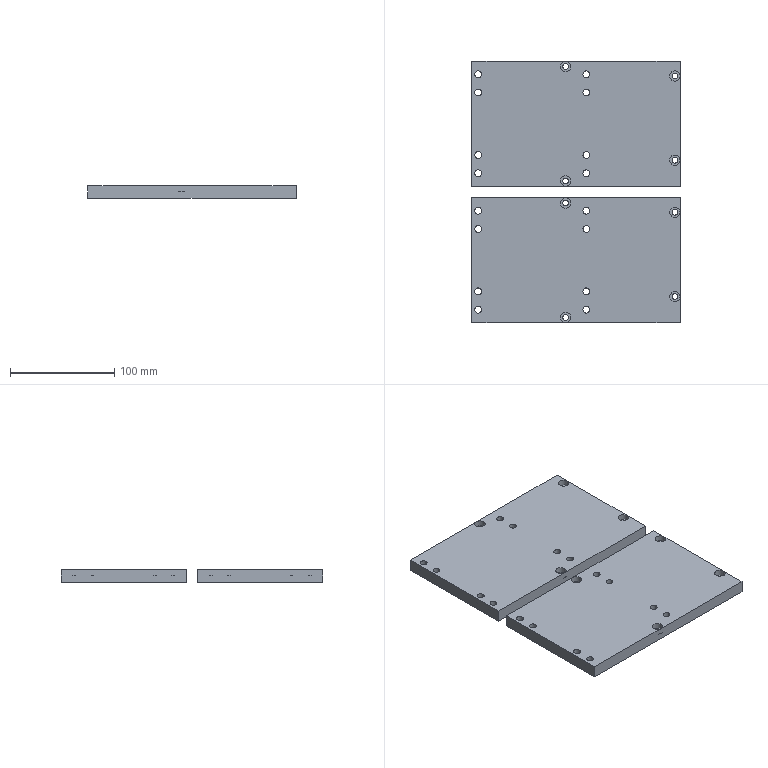Part | 2 solids | 84 faces | box 200 x 251 x 12 mm | volume 558035 mm3 | cylinder 48 | plane 36 | commonest cylinder face diameters 6.6 x16 11 x16 5.5 x8 10 x8